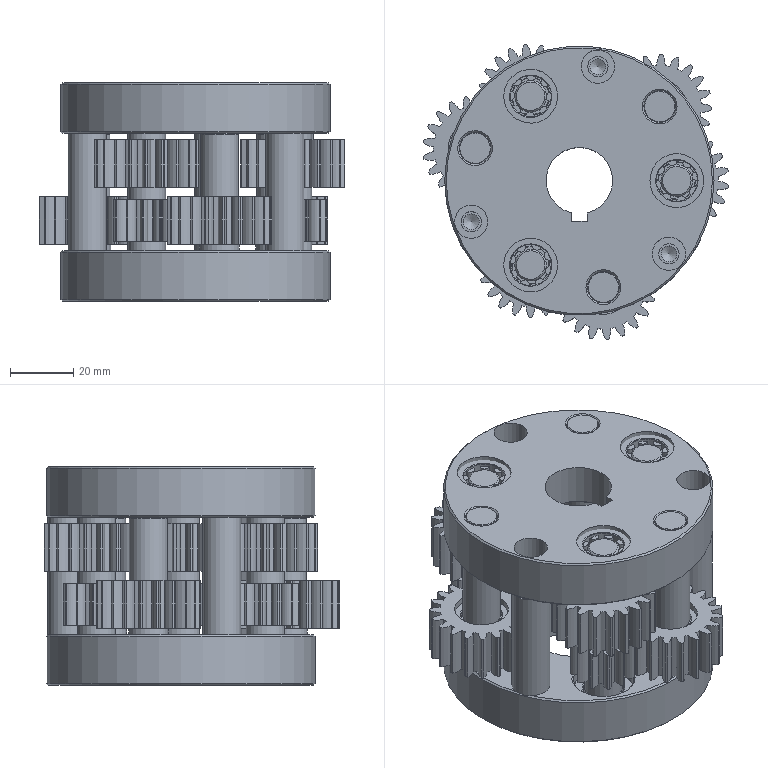Part | NX | features BREP 11 | 33 solids | 1232 faces | box 96.528 x 93.215 x 69 mm | volume 236543 mm3 | cylinder 830 | plane 295 | cone 105 | torus 2 | commonest cylinder face diameters 12 x255 26.248 x120 3 x80 7.2 x72 32.998 x60 33 x60